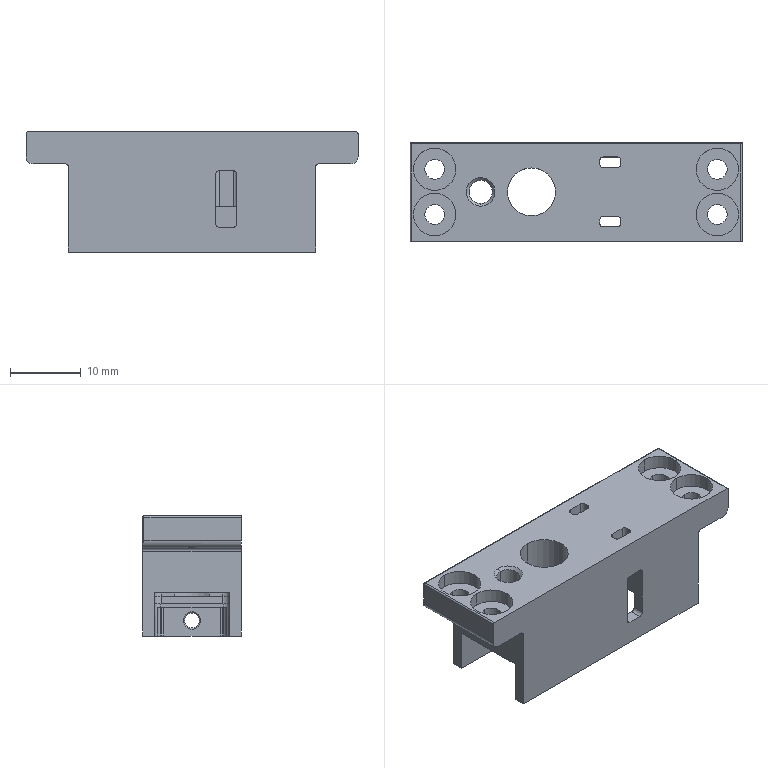NC program | NX | posted with a generic post | part box 47 x 14 x 17 mm
Lines 1 to 1495 of 12912:
N10 G17 G21 G94 G90
(FLOOR_WALL_COPY , TOOL : D63)
N12 T01 M6
N14 G54
N16 G17 G0 G90 X58. Y0. B0. C0. S6500 M3
N18 G43 Z30. H1
N20 Z5.
N22 G94 G1 Z2. F1250.
N24 X55.
N26 X-55.
N28 X-58.
N30 Z5.
N32 G0 Z30.
N34 X58.
N36 Z4.
N38 G1 Z1.
N40 X55.
N42 X-55.
N44 X-58.
N46 Z4.
N48 G0 Z30.
N50 X58.
N52 Z3.
N54 G1 Z0.
N56 X55.
N58 X-55.
N60 X-58.
N62 Z3.
N64 G0 Z30.
N66 M5
(CAVITY_MILL , TOOL : D6)
N68 T09 M6
N70 G54
N72 G17 G0 G90 X27.096 Y-2.483 B0. C0. S9500 M3
N74 G43 Z30. H9
N76 Z0.429
N78 G94 G1 Z-0.571 F1000.
N80 X24.296 Y-0.866
N82 G2 X23.796 Y0. R1.
N84 G1 Y7.002 F2200.
N86 G3 X23.501 Y7.297 R0.295
N88 G1 X21.308
N90 G3 X21.22 Y7.868 R3.82
N92 G1 Y9.997
N94 X20.5
N96 Y7.781
N98 G2 X20.6 Y7. R3.1
N100 G1 Y-7.
N102 G2 X20.3 Y-8.33 R3.1
N104 G1 Y-9.997
N106 X21.02
N108 Y-8.484
N110 G3 X21.308 Y-7.297 R3.82
N112 G1 X23.501
N114 G3 X23.796 Y-7.002 R0.295
N116 G1 Y0.
N118 G2 X24.296 Y0.866 R1.
N120 G1 X27.096 Y2.483
N122 Z0.429
N124 Y-2.483 Z-0.143 F8000.
N126 Z-1.143 F1000.
N128 X24.296 Y-0.866
N130 G2 X23.796 Y0. R1.
N132 G1 Y7.002 F2200.
N134 G3 X23.501 Y7.297 R0.295
N136 G1 X21.308
N138 G3 X21.22 Y7.868 R3.82
N140 G1 Y9.997
N142 X20.5
N144 Y7.781
N146 G2 X20.6 Y7. R3.1
N148 G1 Y-7.
N150 G2 X20.3 Y-8.33 R3.1
N152 G1 Y-9.997
N154 X21.02
N156 Y-8.484
N158 G3 X21.308 Y-7.297 R3.82
N160 G1 X23.501
N162 G3 X23.796 Y-7.002 R0.295
N164 G1 Y0.
N166 G2 X24.296 Y0.866 R1.
N168 G1 X27.096 Y2.483
N170 Z-0.143
N172 Y-2.483 Z-0.714 F8000.
N174 Z-1.714 F1000.
N176 X24.296 Y-0.866
N178 G2 X23.796 Y0. R1.
N180 G1 Y7.002 F2200.
N182 G3 X23.501 Y7.297 R0.296
N184 G1 X21.308
N186 G3 X21.22 Y7.868 R3.82
N188 G1 Y9.997
N190 X20.5
N192 Y7.781
N194 G2 X20.6 Y7. R3.1
N196 G1 Y-7.
N198 G2 X20.5 Y-7.781 R3.1
N200 G1 Y-9.997
N202 X21.22
N204 Y-7.868
N206 G3 X21.308 Y-7.297 R3.82
N208 G1 X23.501
N210 G3 X23.796 Y-7.002 R0.296
N212 G1 Y0.
N214 G2 X24.296 Y0.866 R1.
N216 G1 X27.096 Y2.483
N218 Z-0.714
N220 X27.097 Y-2.483 Z-1.286 F8000.
N222 Z-2.286 F1000.
N224 X24.297 Y-0.866
N226 G2 X23.797 Y0. R1.
N228 G1 Y7.002 F2200.
N230 G3 X23.501 Y7.297 R0.296
N232 G1 X21.308
N234 G3 X21.22 Y7.868 R3.82
N236 G1 Y9.997
N238 X20.5
N240 Y7.781
N242 G2 X20.6 Y7. R3.1
N244 G1 Y-7.
N246 G2 X20.5 Y-7.781 R3.1
N248 G1 Y-9.997
N250 X21.22
N252 Y-7.868
N254 G3 X21.308 Y-7.297 R3.82
N256 G1 X23.501
N258 G3 X23.797 Y-7.002 R0.296
N260 G1 Y0.
N262 G2 X24.297 Y0.866 R1.
N264 G1 X27.097 Y2.483
N266 Z-1.286
N268 Y-2.483 Z-1.857 F8000.
N270 Z-2.857 F1000.
N272 X24.297 Y-0.866
N274 G2 X23.797 Y0. R1.
N276 G1 Y7.002 F2200.
N278 G3 X23.501 Y7.298 R0.296
N280 G1 X21.308
N282 G3 X21.22 Y7.868 R3.82
N284 G1 Y9.998
N286 X20.5
N288 Y7.781
N290 G2 X20.6 Y7. R3.1
N292 G1 Y-7.
N294 G2 X20.5 Y-7.781 R3.1
N296 G1 Y-9.998
N298 X21.22
N300 Y-7.868
N302 G3 X21.308 Y-7.298 R3.82
N304 G1 X23.501
N306 G3 X23.797 Y-7.002 R0.296
N308 G1 Y0.
N310 G2 X24.297 Y0.866 R1.
N312 G1 X27.097 Y2.483
N314 Z-1.857
N316 Y-2.483 Z-2.429 F8000.
N318 Z-3.429 F1000.
N320 X24.297 Y-0.866
N322 G2 X23.797 Y0. R1.
N324 G1 Y7.002 F2200.
N326 G3 X23.501 Y7.298 R0.296
N328 G1 X21.308
N330 G3 X21.22 Y7.868 R3.82
N332 G1 Y9.998
N334 X20.5
N336 Y7.781
N338 G2 X20.6 Y7. R3.1
N340 G1 Y-7.
N342 G2 X20.5 Y-7.781 R3.1
N344 G1 Y-9.998
N346 X21.22
N348 Y-7.868
N350 G3 X21.308 Y-7.298 R3.82
N352 G1 X23.501
N354 G3 X23.797 Y-7.002 R0.296
N356 G1 Y0.
N358 G2 X24.297 Y0.866 R1.
N360 G1 X27.097 Y2.483
N362 Z-2.429
N364 Y-2.483 Z-3. F8000.
N366 Z-4. F1000.
N368 X24.297 Y-0.866
N370 G2 X23.797 Y0. R1.
N372 G1 Y7.002 F2200.
N374 G3 X23.501 Y7.298 R0.296
N376 G1 X21.308
N378 G3 X21.22 Y7.868 R3.82
N380 G1 Y9.998
N382 X20.5
N384 Y7.781
N386 G2 X20.6 Y7. R3.1
N388 G1 Y-7.
N390 G2 X20.5 Y-7.781 R3.1
N392 G1 Y-9.998
N394 X21.22
N396 Y-7.868
N398 G3 X21.308 Y-7.298 R3.82
N400 G1 X23.501
N402 G3 X23.797 Y-7.002 R0.296
N404 G1 Y0.
N406 G2 X24.297 Y0.866 R1.
N408 G1 X27.097 Y2.483
N410 Z-3.
N412 Y-2.483 Z-3.5 F8000.
N414 Z-4.5 F1000.
N416 X24.297 Y-0.866
N418 G2 X23.797 Y0. R1.
N420 G1 Y7.002 F2200.
N422 G3 X23.501 Y7.298 R0.296
N424 G1 X21.308
N426 G3 X21.22 Y7.868 R3.82
N428 G1 Y9.998
N430 X20.5
N432 Y7.781
N434 G2 X20.6 Y7. R3.1
N436 G1 Y-7.
N438 G2 X20.5 Y-7.781 R3.1
N440 G1 Y-9.998
N442 X21.22
N444 Y-7.868
N446 G3 X21.308 Y-7.298 R3.82
N448 G1 X23.501
N450 G3 X23.797 Y-7.002 R0.296
N452 G1 Y0.
N454 G2 X24.297 Y0.866 R1.
N456 G1 X27.097 Y2.483
N458 Z-3.5
N460 Y-2.483 Z-4. F8000.
N462 Z-5. F1000.
N464 X24.297 Y-0.866
N466 G2 X23.797 Y0. R1.
N468 G1 Y7.001 F2200.
N470 G3 X23.501 Y7.298 R0.296
N472 G1 X21.308
N474 G3 X21.22 Y7.868 R3.82
N476 G1 Y9.998
N478 X20.5
N480 Y7.781
N482 G2 X20.6 Y7. R3.1
N484 G1 Y-7.
N486 G2 X20.5 Y-7.781 R3.1
N488 G1 Y-9.998
N490 X21.22
N492 Y-7.868
N494 G3 X21.308 Y-7.298 R3.82
N496 G1 X23.501
N498 G3 X23.797 Y-7.001 R0.296
N500 G1 Y0.
N502 G2 X24.297 Y0.866 R1.
N504 G1 X27.097 Y2.483
N506 Z-4.
N508 Y-2.483 Z-4.5 F8000.
N510 Z-5.5 F1000.
N512 X24.297 Y-0.866
N514 G2 X23.797 Y0. R1.
N516 G1 Y7.001 F2200.
N518 G3 X23.501 Y7.298 R0.297
N520 G1 X21.308
N522 G3 X21.22 Y7.868 R3.82
N524 G1 Y9.998
N526 X20.5
N528 Y7.781
N530 G2 X20.6 Y7. R3.1
N532 G1 Y-7.
N534 G2 X20.5 Y-7.781 R3.1
N536 G1 Y-9.998
N538 X21.22
N540 Y-7.868
N542 G3 X21.308 Y-7.298 R3.82
N544 G1 X23.501
N546 G3 X23.797 Y-7.001 R0.297
N548 G1 Y0.
N550 G2 X24.297 Y0.866 R1.
N552 G1 X27.097 Y2.483
N554 Z-4.5
N556 Y-2.483 Z-5. F8000.
N558 Z-6. F1000.
N560 X24.297 Y-0.866
N562 G2 X23.797 Y0. R1.
N564 G1 Y7.001 F2200.
N566 G3 X23.501 Y7.298 R0.297
N568 G1 X21.308
N570 G3 X21.22 Y7.868 R3.82
N572 G1 Y9.998
N574 X20.5
N576 Y7.781
N578 G2 X20.6 Y7. R3.1
N580 G1 Y-7.
N582 G2 X20.5 Y-7.781 R3.1
N584 G1 Y-9.998
N586 X21.22
N588 Y-7.868
N590 G3 X21.308 Y-7.298 R3.82
N592 G1 X23.501
N594 G3 X23.797 Y-7.001 R0.297
N596 G1 Y0.
N598 G2 X24.297 Y0.866 R1.
N600 G1 X27.097 Y2.483
N602 Z-5.
N604 Y-2.483 Z-5.4 F8000.
N606 Z-6.4 F1000.
N608 X24.297 Y-0.866
N610 G2 X23.797 Y0. R1.
N612 G1 Y7.001 F2200.
N614 G3 X23.501 Y7.298 R0.297
N616 G1 X21.308
N618 G3 X21.22 Y7.868 R3.82
N620 G1 Y9.998
N622 X20.5
N624 Y7.781
N626 G2 X20.6 Y7. R3.1
N628 G1 Y-7.
N630 G2 X20.5 Y-7.781 R3.1
N632 G1 Y-9.998
N634 X21.22
N636 Y-7.868
N638 G3 X21.308 Y-7.298 R3.82
N640 G1 X23.501
N642 G3 X23.797 Y-7.001 R0.297
N644 G1 Y0.
N646 G2 X24.297 Y0.866 R1.
N648 G1 X27.097 Y2.483
N650 Z-5.4
N652 X27.098 Y-2.483 Z-6. F8000.
N654 Z-7. F1000.
N656 X24.298 Y-0.866
N658 G2 X23.798 Y0. R1.
N660 G1 Y7.001 F2200.
N662 G3 X23.501 Y7.298 R0.297
N664 G1 X21.308
N666 G3 X21.22 Y7.868 R3.82
N668 G1 Y9.998
N670 X20.5
N672 Y7.781
N674 G2 X20.6 Y7. R3.1
N676 G1 Y-7.
N678 G2 X20.5 Y-7.781 R3.1
N680 G1 Y-9.998
N682 X21.22
N684 Y-7.868
N686 G3 X21.308 Y-7.298 R3.82
N688 G1 X23.501
N690 G3 X23.798 Y-7.001 R0.297
N692 G1 Y0.
N694 G2 X24.298 Y0.866 R1.
N696 G1 X27.098 Y2.483
N698 Z-6.
N700 Y-2.483 Z-6.55 F8000.
N702 Z-7.55 F1000.
N704 X24.298 Y-0.866
N706 G2 X23.798 Y0. R1.
N708 G1 Y7.001 F2200.
N710 G3 X23.501 Y7.298 R0.297
N712 G1 X21.308
N714 G3 X21.22 Y7.868 R3.82
N716 G1 Y9.998
N718 X20.5
N720 Y7.781
N722 G2 X20.6 Y7. R3.1
N724 G1 Y-7.
N726 G2 X20.5 Y-7.781 R3.1
N728 G1 Y-9.998
N730 X21.22
N732 Y-7.868
N734 G3 X21.308 Y-7.298 R3.82
N736 G1 X23.501
N738 G3 X23.798 Y-7.001 R0.297
N740 G1 Y0.
N742 G2 X24.298 Y0.866 R1.
N744 G1 X27.098 Y2.483
N746 Z-6.55
N748 Y-2.483 Z-7.1 F8000.
N750 Z-8.1 F1000.
N752 X24.298 Y-0.866
N754 G2 X23.798 Y0. R1.
N756 G1 Y7.001 F2200.
N758 G3 X23.501 Y7.298 R0.297
N760 G1 X21.308
N762 G3 X21.22 Y7.868 R3.82
N764 G1 Y9.998
N766 X20.5
N768 Y7.781
N770 G2 X20.6 Y7. R3.1
N772 G1 Y-7.
N774 G2 X20.5 Y-7.781 R3.1
N776 G1 Y-9.998
N778 X21.22
N780 Y-7.868
N782 G3 X21.308 Y-7.298 R3.82
N784 G1 X23.501
N786 G3 X23.798 Y-7.001 R0.297
N788 G1 Y0.
N790 G2 X24.298 Y0.866 R1.
N792 G1 X27.098 Y2.483
N794 Z-7.1
N796 Y-2.483 Z-7.65 F8000.
N798 Z-8.65 F1000.
N800 X24.298 Y-0.866
N802 G2 X23.798 Y0. R1.
N804 G1 Y7.001 F2200.
N806 G3 X23.501 Y7.299 R0.297
N808 G1 X21.308
N810 G3 X21.22 Y7.868 R3.82
N812 G1 Y9.999
N814 X20.5
N816 Y7.781
N818 G2 X20.6 Y7. R3.1
N820 G1 Y-7.
N822 G2 X20.5 Y-7.781 R3.1
N824 G1 Y-9.999
N826 X21.22
N828 Y-7.868
N830 G3 X21.308 Y-7.299 R3.82
N832 G1 X23.501
N834 G3 X23.798 Y-7.001 R0.297
N836 G1 Y0.
N838 G2 X24.298 Y0.866 R1.
N840 G1 X27.098 Y2.483
N842 Z-7.65
N844 Y-2.483 Z-8.2 F8000.
N846 Z-9.2 F1000.
N848 X24.298 Y-0.866
N850 G2 X23.798 Y0. R1.
N852 G1 Y7.001 F2200.
N854 G3 X23.501 Y7.299 R0.298
N856 G1 X21.308
N858 G3 X21.22 Y7.868 R3.82
N860 G1 Y9.999
N862 X20.5
N864 Y7.781
N866 G2 X20.6 Y7. R3.1
N868 G1 Y-7.
N870 G2 X20.5 Y-7.781 R3.1
N872 G1 Y-9.999
N874 X21.22
N876 Y-7.868
N878 G3 X21.308 Y-7.299 R3.82
N880 G1 X23.501
N882 G3 X23.798 Y-7.001 R0.298
N884 G1 Y0.
N886 G2 X24.298 Y0.866 R1.
N888 G1 X27.098 Y2.483
N890 Z-8.2
N892 Y-2.483 Z-8.75 F8000.
N894 Z-9.75 F1000.
N896 X24.298 Y-0.866
N898 G2 X23.798 Y0. R1.
N900 G1 Y7.001 F2200.
N902 G3 X23.501 Y7.299 R0.298
N904 G1 X21.308
N906 G3 X21.22 Y7.868 R3.82
N908 G1 Y9.999
N910 X20.5
N912 Y7.781
N914 G2 X20.6 Y7. R3.1
N916 G1 Y-7.
N918 G2 X20.5 Y-7.781 R3.1
N920 G1 Y-9.999
N922 X21.22
N924 Y-7.868
N926 G3 X21.308 Y-7.299 R3.82
N928 G1 X23.501
N930 G3 X23.798 Y-7.001 R0.298
N932 G1 Y0.
N934 G2 X24.298 Y0.866 R1.
N936 G1 X27.098 Y2.483
N938 Z-8.75
N940 Y-2.483 Z-9.3 F8000.
N942 Z-10.3 F1000.
N944 X24.298 Y-0.866
N946 G2 X23.798 Y0. R1.
N948 G1 Y7.001 F2200.
N950 G3 X23.5 Y7.299 R0.298
N952 G1 X21.308
N954 G3 X21.22 Y7.868 R3.82
N956 G1 Y9.999
N958 X20.5
N960 Y7.781
N962 G2 X20.6 Y7. R3.1
N964 G1 Y-7.
N966 G2 X20.5 Y-7.781 R3.1
N968 G1 Y-9.999
N970 X21.22
N972 Y-7.868
N974 G3 X21.308 Y-7.299 R3.82
N976 G1 X23.5
N978 G3 X23.798 Y-7.001 R0.298
N980 G1 Y0.
N982 G2 X24.298 Y0.866 R1.
N984 G1 X27.098 Y2.483
N986 Z-9.3
N988 Y-2.483 Z-9.85 F8000.
N990 Z-10.85 F1000.
N992 X24.298 Y-0.866
N994 G2 X23.798 Y0. R1.
N996 G1 Y7.001 F2200.
N998 G3 X23.5 Y7.299 R0.298
N1000 G1 X21.308
N1002 G3 X21.22 Y7.868 R3.82
N1004 G1 Y9.999
N1006 X20.5
N1008 Y7.781
N1010 G2 X20.6 Y7. R3.1
N1012 G1 Y-7.
N1014 G2 X20.5 Y-7.781 R3.1
N1016 G1 Y-9.999
N1018 X21.22
N1020 Y-7.868
N1022 G3 X21.308 Y-7.299 R3.82
N1024 G1 X23.5
N1026 G3 X23.798 Y-7.001 R0.298
N1028 G1 Y0.
N1030 G2 X24.298 Y0.866 R1.
N1032 G1 X27.098 Y2.483
N1034 Z-9.85
N1036 X27.099 Y-2.483 Z-10.4 F8000.
N1038 Z-11.4 F1000.
N1040 X24.299 Y-0.866
N1042 G2 X23.799 Y0. R1.
N1044 G1 Y7.001 F2200.
N1046 G3 X23.5 Y7.299 R0.298
N1048 G1 X21.308
N1050 G3 X21.22 Y7.868 R3.82
N1052 G1 Y9.999
N1054 X20.5
N1056 Y7.781
N1058 G2 X20.6 Y7. R3.1
N1060 G1 Y-7.
N1062 G2 X20.5 Y-7.781 R3.1
N1064 G1 Y-9.999
N1066 X21.22
N1068 Y-7.868
N1070 G3 X21.308 Y-7.299 R3.82
N1072 G1 X23.5
N1074 G3 X23.799 Y-7.001 R0.298
N1076 G1 Y0.
N1078 G2 X24.299 Y0.866 R1.
N1080 G1 X27.099 Y2.483
N1082 Z-10.4
N1084 Y-2.483 Z-10.5 F8000.
N1086 Z-11.5 F1000.
N1088 X24.299 Y-0.866
N1090 G2 X23.799 Y0. R1.
N1092 G1 Y7.001 F2200.
N1094 G3 X23.5 Y7.299 R0.298
N1096 G1 X21.308
N1098 G3 X21.22 Y7.868 R3.82
N1100 G1 Y9.999
N1102 X20.5
N1104 Y7.781
N1106 G2 X20.6 Y7. R3.1
N1108 G1 Y-7.
N1110 G2 X20.5 Y-7.781 R3.1
N1112 G1 Y-9.999
N1114 X21.22
N1116 Y-7.868
N1118 G3 X21.308 Y-7.299 R3.82
N1120 G1 X23.5
N1122 G3 X23.799 Y-7.001 R0.298
N1124 G1 Y0.
N1126 G2 X24.299 Y0.866 R1.
N1128 G1 X27.099 Y2.483
N1130 Z-10.5
N1132 Y-2.483 Z-10.95 F8000.
N1134 Z-11.95 F1000.
N1136 X24.299 Y-0.866
N1138 G2 X23.799 Y0. R1.
N1140 G1 Y7.001 F2200.
N1142 G3 X23.5 Y7.299 R0.298
N1144 G1 X21.308
N1146 G3 X21.22 Y7.868 R3.82
N1148 G1 Y9.999
N1150 X20.5
N1152 Y7.781
N1154 G2 X20.6 Y7. R3.1
N1156 G1 Y-7.
N1158 G2 X20.5 Y-7.781 R3.1
N1160 G1 Y-9.999
N1162 X21.22
N1164 Y-7.868
N1166 G3 X21.308 Y-7.299 R3.82
N1168 G1 X23.5
N1170 G3 X23.799 Y-7.001 R0.298
N1172 G1 Y0.
N1174 G2 X24.299 Y0.866 R1.
N1176 G1 X27.099 Y2.483
N1178 Z-10.95
N1180 Y-2.483 Z-11.4 F8000.
N1182 Z-12.4 F1000.
N1184 X24.299 Y-0.866
N1186 G2 X23.799 Y0. R1.
N1188 G1 Y7.001 F2200.
N1190 G3 X23.5 Y7.299 R0.298
N1192 G1 X21.632
N1194 G3 X21.42 Y8.254 R3.878
N1196 G1 Y9.999
N1198 X20.7
N1200 Y8.122
N1202 G2 X20.928 Y7.002 R3.158
N1204 G1 X20.923 Y6.542
N1206 Y-6.542
N1208 X20.928 Y-7.002
N1210 G2 X20.7 Y-8.128 R3.151
N1212 G1 Y-9.999
N1214 X21.42
N1216 Y-8.26
N1218 G3 X21.633 Y-7.299 R3.871
N1220 G1 X23.5
N1222 G3 X23.799 Y-7.001 R0.298
N1224 G1 Y0.
N1226 G2 X24.299 Y0.866 R1.
N1228 G1 X27.099 Y2.483
N1230 Z-11.4
N1232 G0 Z30.
N1234 X-27.096 Y-2.483
N1236 Z0.429
N1238 G1 Z-0.571 F1000.
N1240 X-24.296 Y-0.866
N1242 G3 X-23.796 Y0. R1.
N1244 G1 X-21.096
N1246 Y-0.799 F2200.
N1248 G2 X-19.74 Y0. R5.8
N1250 X-21.096 Y0.799 R5.8
N1252 G1 Y0.
N1254 X-23.796
N1256 Y-7.002
N1258 G3 X-23.501 Y-7.297 R0.295
N1260 G1 X-21.308
N1262 G3 X-21.22 Y-7.868 R3.82
N1264 G1 Y-9.997
N1266 X-20.5
N1268 Y-7.781
N1270 G2 X-20.6 Y-7. R3.1
N1272 G1 Y-5.35
N1274 G2 X-17.5 Y-2.25 R3.1
N1276 G1 X7.606
N1278 G2 X8.387 Y-2.15 R3.1
N1280 G1 X9.162
N1282 G2 X9.433 Y-2.031 R3.1
N1284 X10.1 Y-1.575 R3.24
N1286 G1 Y1.617
N1288 X10.055 Y1.639
N1290 X10.039 Y1.607
N1292 G2 X9.433 Y2.031 R3.24
N1294 X9.162 Y2.15 R3.1
N1296 G1 X8.387
N1298 G2 X7.606 Y2.25 R3.1
N1300 G1 X-17.5
N1302 G2 X-20.6 Y5.35 R3.1
N1304 G1 Y7.
N1306 G2 X-20.5 Y7.781 R3.1
N1308 G1 Y9.997
N1310 X-21.22
N1312 Y7.868
N1314 G3 X-21.308 Y7.297 R3.82
N1316 G1 X-23.501
N1318 G3 X-23.796 Y7.002 R0.295
N1320 G1 Y0.
N1322 G2 X-24.296 Y-0.866 R1.
N1324 G1 X-27.096 Y-2.483
N1326 Z0.429
N1328 Z-0.143 F8000.
N1330 Z-1.143 F1000.
N1332 X-24.296 Y-0.866
N1334 G3 X-23.796 Y0. R1.
N1336 G1 X-21.096
N1338 Y-0.8 F2200.
N1340 G2 X-19.74 Y0. R5.8
N1342 X-21.096 Y0.8 R5.8
N1344 G1 Y0.
N1346 X-23.796
N1348 Y-7.002
N1350 G3 X-23.501 Y-7.297 R0.295
N1352 G1 X-21.308
N1354 G3 X-21.22 Y-7.868 R3.82
N1356 G1 Y-9.997
N1358 X-20.5
N1360 Y-7.781
N1362 G2 X-20.6 Y-7. R3.1
N1364 G1 Y-5.35
N1366 G2 X-17.5 Y-2.25 R3.1
N1368 G1 X7.606
N1370 G2 X8.387 Y-2.15 R3.1
N1372 G1 X9.162
N1374 G2 X9.433 Y-2.031 R3.1
N1376 X10.1 Y-1.575 R3.24
N1378 G1 Y1.617
N1380 X10.055 Y1.639
N1382 X10.039 Y1.607
N1384 G2 X9.433 Y2.031 R3.24
N1386 X9.162 Y2.15 R3.1
N1388 G1 X8.387
N1390 G2 X7.606 Y2.25 R3.1
N1392 G1 X-17.5
N1394 G2 X-20.6 Y5.35 R3.1
N1396 G1 Y7.
N1398 G2 X-20.5 Y7.781 R3.1
N1400 G1 Y9.997
N1402 X-21.22
N1404 Y7.868
N1406 G3 X-21.308 Y7.297 R3.82
N1408 G1 X-23.501
N1410 G3 X-23.796 Y7.002 R0.295
N1412 G1 Y0.
N1414 G2 X-24.296 Y-0.866 R1.
N1416 G1 X-27.096 Y-2.483
N1418 Z-0.143
N1420 Z-0.714 F8000.
N1422 Z-1.714 F1000.
N1424 X-24.296 Y-0.866
N1426 G3 X-23.796 Y0. R1.
N1428 G1 X-21.096
N1430 Y-0.8 F2200.
N1432 G2 X-19.74 Y0. R5.8
N1434 X-21.096 Y0.8 R5.8
N1436 G1 Y0.
N1438 X-23.796
N1440 Y-7.002
N1442 G3 X-23.501 Y-7.297 R0.296
N1444 G1 X-21.308
N1446 G3 X-21.22 Y-7.868 R3.82
N1448 G1 Y-9.997
N1450 X-20.5
N1452 Y-7.781
N1454 G2 X-20.6 Y-7. R3.1
N1456 G1 Y-5.35
N1458 G2 X-17.5 Y-2.25 R3.1
N1460 G1 X7.606
N1462 G2 X8.387 Y-2.15 R3.1
N1464 G1 X9.162
N1466 G2 X9.433 Y-2.031 R3.1
N1468 X10.1 Y-1.575 R3.24
N1470 G1 Y1.617
N1472 X10.055 Y1.639
N1474 X10.039 Y1.607
N1476 G2 X9.433 Y2.031 R3.24
N1478 X9.162 Y2.15 R3.1
N1480 G1 X8.387
N1482 G2 X7.606 Y2.25 R3.1
N1484 G1 X-17.5
N1486 G2 X-20.6 Y5.35 R3.1
N1488 G1 Y7.
N1490 G2 X-20.5 Y7.781 R3.1
N1492 G1 Y9.997
N1494 X-21.22
N1496 Y7.868
N1498 G3 X-21.308 Y7.297 R3.82
N1500 G1 X-23.501
N1502 G3 X-23.796 Y7.002 R0.296
N1504 G1 Y0.
N1506 G2 X-24.296 Y-0.866 R1.
N1508 G1 X-27.096 Y-2.483
N1510 Z-0.714
N1512 X-27.097 Z-1.286 F8000.
N1514 Z-2.286 F1000.
N1516 X-24.297 Y-0.866
N1518 G3 X-23.797 Y0. R1.
N1520 G1 X-21.097
N1522 Y-0.8 F2200.
N1524 G2 X-19.74 Y0. R5.8
N1526 X-21.097 Y0.8 R5.8
N1528 G1 Y0.
N1530 X-23.797
N1532 Y-7.002
N1534 G3 X-23.501 Y-7.297 R0.296
N1536 G1 X-21.308
N1538 G3 X-21.22 Y-7.868 R3.82
N1540 G1 Y-9.997
N1542 X-20.5
N1544 Y-7.781
N1546 G2 X-20.6 Y-7. R3.1
N1548 G1 Y-5.35
N1550 G2 X-17.5 Y-2.25 R3.1
N1552 G1 X7.606
N1554 G2 X8.387 Y-2.15 R3.1
N1556 G1 X9.162
N1558 G2 X9.433 Y-2.031 R3.1
N1560 X10.1 Y-1.574 R3.241
N1562 G1 Y1.617
N1564 X10.055 Y1.639
N1566 X10.039 Y1.607
N1568 G2 X9.433 Y2.031 R3.24
N1570 X9.162 Y2.15 R3.1
N1572 G1 X8.387
N1574 G2 X7.606 Y2.25 R3.1
N1576 G1 X-17.5
N1578 G2 X-20.6 Y5.35 R3.1
N1580 G1 Y7.
N1582 G2 X-20.5 Y7.781 R3.1
N1584 G1 Y9.997
N1586 X-21.22
N1588 Y7.868
N1590 G3 X-21.308 Y7.297 R3.82
N1592 G1 X-23.501
N1594 G3 X-23.797 Y7.002 R0.296
N1596 G1 Y0.
N1598 G2 X-24.297 Y-0.866 R1.
N1600 G1 X-27.097 Y-2.483
N1602 Z-1.286
N1604 Z-1.857 F8000.
N1606 Z-2.857 F1000.
N1608 X-24.297 Y-0.866
N1610 G3 X-23.797 Y0. R1.
N1612 G1 X-21.097
N1614 Y-0.8 F2200.
N1616 G2 X-19.74 Y0. R5.8
N1618 X-21.097 Y0.8 R5.8
N1620 G1 Y0.
N1622 X-23.797
N1624 Y-7.002
N1626 G3 X-23.501 Y-7.298 R0.296
N1628 G1 X-21.308
N1630 G3 X-21.22 Y-7.868 R3.82
N1632 G1 Y-9.998
N1634 X-20.5
N1636 Y-7.781
N1638 G2 X-20.6 Y-7. R3.1
N1640 G1 Y-5.35
N1642 G2 X-17.5 Y-2.25 R3.1
N1644 G1 X7.606
N1646 G2 X8.387 Y-2.15 R3.1
N1648 G1 X9.162
N1650 G2 X9.433 Y-2.031 R3.1
N1652 X10.1 Y-1.575 R3.24
N1654 G1 Y1.617
N1656 X10.055 Y1.639
N1658 X10.039 Y1.607
N1660 G2 X9.433 Y2.031 R3.24
N1662 X9.162 Y2.15 R3.1
N1664 G1 X8.387
N1666 G2 X7.606 Y2.25 R3.1
N1668 G1 X-17.5
N1670 G2 X-20.6 Y5.35 R3.1
N1672 G1 Y7.
N1674 G2 X-20.5 Y7.781 R3.1
N1676 G1 Y9.998
N1678 X-21.22
N1680 Y7.868
N1682 G3 X-21.308 Y7.298 R3.82
N1684 G1 X-23.501
N1686 G3 X-23.797 Y7.002 R0.296
N1688 G1 Y0.
N1690 G2 X-24.297 Y-0.866 R1.
N1692 G1 X-27.097 Y-2.483
N1694 Z-1.857
N1696 Z-2.429 F8000.
N1698 Z-3.429 F1000.
N1700 X-24.297 Y-0.866
N1702 G3 X-23.797 Y0. R1.
N1704 G1 X-21.097
N1706 Y-0.8 F2200.
N1708 G2 X-19.74 Y0. R5.8
N1710 X-21.097 Y0.8 R5.8
N1712 G1 Y0.
N1714 X-23.797
N1716 Y-7.002
N1718 G3 X-23.501 Y-7.298 R0.296
N1720 G1 X-21.308
N1722 G3 X-21.22 Y-7.868 R3.82
N1724 G1 Y-9.998
N1726 X-20.5
N1728 Y-7.781
N1730 G2 X-20.6 Y-7. R3.1
N1732 G1 Y-5.35
N1734 G2 X-17.5 Y-2.25 R3.1
N1736 G1 X7.606
N1738 G2 X8.387 Y-2.15 R3.1
N1740 G1 X9.162
N1742 G2 X9.433 Y-2.031 R3.1
N1744 X10.1 Y-1.575 R3.241
N1746 G1 Y1.617
N1748 X10.055 Y1.639
N1750 X10.039 Y1.607
N1752 G2 X9.433 Y2.031 R3.24
N1754 X9.162 Y2.15 R3.1
N1756 G1 X8.387
N1758 G2 X7.606 Y2.25 R3.1
N1760 G1 X-17.5
N1762 G2 X-20.6 Y5.35 R3.1
N1764 G1 Y7.
N1766 G2 X-20.5 Y7.781 R3.1
N1768 G1 Y9.998
N1770 X-21.22
N1772 Y7.868
N1774 G3 X-21.308 Y7.298 R3.82
N1776 G1 X-23.501
N1778 G3 X-23.797 Y7.002 R0.296
N1780 G1 Y0.
N1782 G2 X-24.297 Y-0.866 R1.
N1784 G1 X-27.097 Y-2.483
N1786 Z-2.429
N1788 Z-3. F8000.
N1790 Z-4. F1000.
N1792 X-24.297 Y-0.866
N1794 G3 X-23.797 Y0. R1.
N1796 G1 X-21.097
N1798 Y-0.8 F2200.
N1800 G2 X-19.74 Y0. R5.8
N1802 X-21.097 Y0.8 R5.8
N1804 G1 Y0.
N1806 X-23.797
N1808 Y-7.002
N1810 G3 X-23.501 Y-7.298 R0.296
N1812 G1 X-21.308
N1814 G3 X-21.22 Y-7.868 R3.82
N1816 G1 Y-9.998
N1818 X-20.5
N1820 Y-7.781
N1822 G2 X-20.6 Y-7. R3.1
N1824 G1 Y-5.35
N1826 G2 X-17.5 Y-2.25 R3.1
N1828 G1 X7.606
N1830 G2 X8.387 Y-2.15 R3.1
N1832 G1 X9.162
N1834 G2 X9.433 Y-2.031 R3.1
N1836 X10.1 Y-1.574 R3.241
N1838 G1 Y1.617
N1840 X10.055 Y1.639
N1842 X10.039 Y1.607
N1844 G2 X9.433 Y2.031 R3.24
N1846 X9.162 Y2.15 R3.1
N1848 G1 X8.387
N1850 G2 X7.606 Y2.25 R3.1
N1852 G1 X-17.5
N1854 G2 X-20.6 Y5.35 R3.1
N1856 G1 Y7.
N1858 G2 X-20.5 Y7.781 R3.1
N1860 G1 Y9.998
N1862 X-21.22
N1864 Y7.868
N1866 G3 X-21.308 Y7.298 R3.82
N1868 G1 X-23.501
N1870 G3 X-23.797 Y7.002 R0.296
N1872 G1 Y0.
N1874 G2 X-24.297 Y-0.866 R1.
N1876 G1 X-27.097 Y-2.483
N1878 Z-3.
N1880 Z-3.5 F8000.
N1882 Z-4.5 F1000.
N1884 X-24.297 Y-0.866
N1886 G3 X-23.797 Y0. R1.
N1888 G1 X-21.097
N1890 Y-0.8 F2200.
N1892 G2 X-19.74 Y0. R5.8
N1894 X-21.097 Y0.8 R5.8
N1896 G1 Y0.
N1898 X-23.797
N1900 Y-7.002
N1902 G3 X-23.501 Y-7.298 R0.296
N1904 G1 X-21.308
N1906 G3 X-21.22 Y-7.868 R3.82
N1908 G1 Y-9.998
N1910 X-20.5
N1912 Y-7.781
N1914 G2 X-20.6 Y-7. R3.1
N1916 G1 Y-5.35
N1918 G2 X-17.5 Y-2.25 R3.1
N1920 G1 X7.6
N1922 Y2.25
N1924 X-17.5
N1926 G2 X-20.6 Y5.35 R3.1
N1928 G1 Y7.
N1930 G2 X-20.5 Y7.781 R3.1
N1932 G1 Y9.998
N1934 X-21.22
N1936 Y7.868
N1938 G3 X-21.308 Y7.298 R3.82
N1940 G1 X-23.501
N1942 G3 X-23.797 Y7.002 R0.296
N1944 G1 Y0.
N1946 G2 X-24.297 Y-0.866 R1.
N1948 G1 X-27.097 Y-2.483
N1950 Z-3.5
N1952 X5.572 Y2.25 F8000.
N1954 X2.7 Z-3.651 F1000.
N1956 Y-2.25 Z-3.886
N1958 X7.6 Z-4.143
N1960 Y2.25 Z-4.379
N1962 X2.7 Z-4.636
N1964 Y-2.25 Z-4.872
N1966 X5.15 Z-5.
N1968 X7.6 F2200.
N1970 Y2.25
N1972 X2.7
N1974 Y-2.25
N1976 X5.15
N1978 G3 X6.016 Y-1.75 R1.
N1980 G1 Z-4.
N1982 X5.572 Y2.25 F8000.
N1984 X2.7 Z-4.151 F1000.
N1986 Y-2.25 Z-4.386
N1988 X7.6 Z-4.643
N1990 Y2.25 Z-4.879
N1992 X2.7 Z-5.136
N1994 Y-2.25 Z-5.372
N1996 X5.15 Z-5.5
N1998 X7.6 F2200.
N2000 Y2.25
N2002 X2.7
N2004 Y-2.25
N2006 X5.15
N2008 G3 X6.016 Y-1.75 R1.
N2010 G1 Z-4.5
N2012 X5.572 Y2.25 F8000.
N2014 X2.7 Z-4.651 F1000.
N2016 Y-2.25 Z-4.886
N2018 X7.6 Z-5.143
N2020 Y2.25 Z-5.379
N2022 X2.7 Z-5.636
N2024 Y-2.25 Z-5.872
N2026 X5.15 Z-6.
N2028 X7.6 F2200.
N2030 Y2.25
N2032 X2.7
N2034 Y-2.25
N2036 X5.15
N2038 G3 X6.016 Y-1.75 R1.
N2040 G1 Z-5.
N2042 X3.664 Y2.25 F8000.
N2044 X2.7 Z-5.051 F1000.
N2046 Y-2.25 Z-5.286
N2048 X7.6 Z-5.543
N2050 Y2.25 Z-5.779
N2052 X2.7 Z-6.036
N2054 Y-2.25 Z-6.272
N2056 X5.15 Z-6.4
N2058 X7.6 F2200.
N2060 Y2.25
N2062 X2.7
N2064 Y-2.25
N2066 X5.15
N2068 G3 X6.016 Y-1.75 R1.
N2070 G1 Z-5.4
N2072 G0 Z30.
N2074 X-27.097 Y-2.483
N2076 Z-4.
N2078 G1 Z-5. F1000.
N2080 X-24.297 Y-0.866
N2082 G3 X-23.797 Y0. R1.
N2084 G1 X-21.097
N2086 Y-0.8 F2200.
N2088 G2 X-19.74 Y0. R5.8
N2090 X-21.097 Y0.8 R5.8
N2092 G1 Y0.
N2094 X-23.797
N2096 Y-7.001
N2098 G3 X-23.501 Y-7.298 R0.296
N2100 G1 X-21.308
N2102 G3 X-21.22 Y-7.868 R3.82
N2104 G1 Y-9.998
N2106 X-20.5
N2108 Y-7.781
N2110 G2 X-20.6 Y-7. R3.1
N2112 G1 Y-5.35
N2114 G2 X-17.5 Y-2.25 R3.1
N2116 G1 X-5.1
N2118 Y2.25
N2120 X-17.5
N2122 G2 X-20.6 Y5.35 R3.1
N2124 G1 Y7.
N2126 G2 X-20.5 Y7.781 R3.1
N2128 G1 Y9.998
N2130 X-21.22
N2132 Y7.868
N2134 G3 X-21.308 Y7.298 R3.82
N2136 G1 X-23.501
N2138 G3 X-23.797 Y7.001 R0.296
N2140 G1 Y0.
N2142 G2 X-24.297 Y-0.866 R1.
N2144 G1 X-27.097 Y-2.483
N2146 Z-4.
N2148 Z-4.5 F8000.
N2150 Z-5.5 F1000.
N2152 X-24.297 Y-0.866
N2154 G3 X-23.797 Y0. R1.
N2156 G1 X-21.097
N2158 Y-0.8 F2200.
N2160 G2 X-19.74 Y0. R5.8
N2162 X-21.097 Y0.8 R5.8
N2164 G1 Y0.
N2166 X-23.797
N2168 Y-7.001
N2170 G3 X-23.501 Y-7.298 R0.297
N2172 G1 X-21.308
N2174 G3 X-21.22 Y-7.868 R3.82
N2176 G1 Y-9.998
N2178 X-20.5
N2180 Y-7.781
N2182 G2 X-20.6 Y-7. R3.1
N2184 G1 Y-5.35
N2186 G2 X-17.5 Y-2.25 R3.1
N2188 G1 X-5.1
N2190 Y2.25
N2192 X-17.5
N2194 G2 X-20.6 Y5.35 R3.1
N2196 G1 Y7.
N2198 G2 X-20.5 Y7.781 R3.1
N2200 G1 Y9.998
N2202 X-21.22
N2204 Y7.868
N2206 G3 X-21.308 Y7.298 R3.82
N2208 G1 X-23.501
N2210 G3 X-23.797 Y7.001 R0.297
N2212 G1 Y0.
N2214 G2 X-24.297 Y-0.866 R1.
N2216 G1 X-27.097 Y-2.483
N2218 Z-4.5
N2220 Z-5. F8000.
N2222 Z-6. F1000.
N2224 X-24.297 Y-0.866
N2226 G3 X-23.797 Y0. R1.
N2228 G1 X-21.097
N2230 Y-0.8 F2200.
N2232 G2 X-19.74 Y0. R5.8
N2234 X-21.097 Y0.8 R5.8
N2236 G1 Y0.
N2238 X-23.797
N2240 Y-7.001
N2242 G3 X-23.501 Y-7.298 R0.297
N2244 G1 X-21.308
N2246 G3 X-21.22 Y-7.868 R3.82
N2248 G1 Y-9.998
N2250 X-20.5
N2252 Y-7.781
N2254 G2 X-20.6 Y-7. R3.1
N2256 G1 Y-5.35
N2258 G2 X-17.5 Y-2.25 R3.1
N2260 G1 X-6.095
N2262 G2 X-5.495 Y-0.593 R3.1
N2264 G3 X-5.495 Y0.593 R1.
N2266 G2 X-6.095 Y2.25 R3.1
N2268 G1 X-17.5
N2270 G2 X-20.6 Y5.35 R3.1
N2272 G1 Y7.
N2274 G2 X-20.5 Y7.781 R3.1
N2276 G1 Y9.998
N2278 X-21.22
N2280 Y7.868
N2282 G3 X-21.308 Y7.298 R3.82
N2284 G1 X-23.501
N2286 G3 X-23.797 Y7.001 R0.297
N2288 G1 Y0.
N2290 G2 X-24.297 Y-0.866 R1.
N2292 G1 X-27.097 Y-2.483
N2294 Z-5.
N2296 X-21.1 Y10.598 Z-5.4 F8000.
N2298 Z-6.4 F1000.
N2300 X-20.61 Y10.065
N2302 G2 X-20.86 Y9.998 R0.5
N2304 G1 X-21.22 F2200.
N2306 Y7.868
N2308 G3 X-21.308 Y7.298 R3.82
N2310 G1 X-23.501
N2312 G3 X-23.797 Y7.001 R0.297
N2314 G1 Y-7.001
N2316 G3 X-23.501 Y-7.298 R0.297
N2318 G1 X-21.308
N2320 G3 X-21.22 Y-7.868 R3.82
N2322 G1 Y-9.998
N2324 X-20.5
N2326 Y-7.781
N2328 G2 X-20.6 Y-7. R3.1
N2330 G1 Y7.
N2332 G2 X-20.5 Y7.781 R3.1
N2334 G1 Y9.998
N2336 X-20.86
N2338 G2 X-21.726 Y10.498 R1.
N2340 G1 X-21.784 Y10.598
N2342 Z-5.4
N2344 X-21.1 Z-6. F8000.
N2346 Z-7. F1000.
N2348 X-20.61 Y10.065
N2350 G2 X-20.86 Y9.998 R0.5
N2352 G1 X-21.22 F2200.
N2354 Y7.868
N2356 G3 X-21.308 Y7.298 R3.82
N2358 G1 X-23.501
N2360 G3 X-23.798 Y7.001 R0.297
N2362 G1 Y-7.001
N2364 G3 X-23.501 Y-7.298 R0.297
N2366 G1 X-21.308
N2368 G3 X-21.22 Y-7.868 R3.82
N2370 G1 Y-9.998
N2372 X-20.5
N2374 Y-7.781
N2376 G2 X-20.6 Y-7. R3.1
N2378 G1 Y7.
N2380 G2 X-20.5 Y7.781 R3.1
N2382 G1 Y9.998
N2384 X-20.86
N2386 G2 X-21.726 Y10.498 R1.
N2388 G1 X-21.784 Y10.598
N2390 Z-6.
N2392 X-21.1 Z-6.55 F8000.
N2394 Z-7.55 F1000.
N2396 X-20.61 Y10.065
N2398 G2 X-20.86 Y9.998 R0.5
N2400 G1 X-21.22 F2200.
N2402 Y7.868
N2404 G3 X-21.308 Y7.298 R3.82
N2406 G1 X-23.501
N2408 G3 X-23.798 Y7.001 R0.297
N2410 G1 Y-7.001
N2412 G3 X-23.501 Y-7.298 R0.297
N2414 G1 X-21.308
N2416 G3 X-21.22 Y-7.868 R3.82
N2418 G1 Y-9.998
N2420 X-20.5
N2422 Y-7.781
N2424 G2 X-20.6 Y-7. R3.1
N2426 G1 Y7.
N2428 G2 X-20.5 Y7.781 R3.1
N2430 G1 Y9.998
N2432 X-20.86
N2434 G2 X-21.726 Y10.498 R1.
N2436 G1 X-21.784 Y10.598
N2438 Z-6.55
N2440 X-21.1 Z-7.1 F8000.
N2442 Z-8.1 F1000.
N2444 X-20.61 Y10.065
N2446 G2 X-20.86 Y9.998 R0.5
N2448 G1 X-21.22 F2200.
N2450 Y7.868
N2452 G3 X-21.308 Y7.298 R3.82
N2454 G1 X-23.501
N2456 G3 X-23.798 Y7.001 R0.297
N2458 G1 Y-7.001
N2460 G3 X-23.501 Y-7.298 R0.297
N2462 G1 X-21.308
N2464 G3 X-21.22 Y-7.868 R3.82
N2466 G1 Y-9.998
N2468 X-20.5
N2470 Y-7.781
N2472 G2 X-20.6 Y-7. R3.1
N2474 G1 Y7.
N2476 G2 X-20.5 Y7.781 R3.1
N2478 G1 Y9.998
N2480 X-20.86
N2482 G2 X-21.726 Y10.498 R1.
N2484 G1 X-21.784 Y10.598
N2486 Z-7.1
N2488 X-21.1 Y10.599 Z-7.65 F8000.
N2490 Z-8.65 F1000.
N2492 X-20.61 Y10.066
N2494 G2 X-20.86 Y9.999 R0.5
N2496 G1 X-21.22 F2200.
N2498 Y7.868
N2500 G3 X-21.308 Y7.299 R3.82
N2502 G1 X-23.501
N2504 G3 X-23.798 Y7.001 R0.297
N2506 G1 Y-7.001
N2508 G3 X-23.501 Y-7.299 R0.297
N2510 G1 X-21.308
N2512 G3 X-21.22 Y-7.868 R3.82
N2514 G1 Y-9.999
N2516 X-20.5
N2518 Y-7.781
N2520 G2 X-20.6 Y-7. R3.1
N2522 G1 Y7.
N2524 G2 X-20.5 Y7.781 R3.1
N2526 G1 Y9.999
N2528 X-20.86
N2530 G2 X-21.726 Y10.499 R1.
N2532 G1 X-21.784 Y10.599
N2534 Z-7.65
N2536 X-21.1 Z-8.2 F8000.
N2538 Z-9.2 F1000.
N2540 X-20.61 Y10.066
N2542 G2 X-20.86 Y9.999 R0.5
N2544 G1 X-21.22 F2200.
N2546 Y7.868
N2548 G3 X-21.308 Y7.299 R3.82
N2550 G1 X-23.501
N2552 G3 X-23.798 Y7.001 R0.298
N2554 G1 Y-7.001
N2556 G3 X-23.501 Y-7.299 R0.298
N2558 G1 X-21.308
N2560 G3 X-21.22 Y-7.868 R3.82
N2562 G1 Y-9.999
N2564 X-20.5
N2566 Y-7.781
N2568 G2 X-20.6 Y-7. R3.1
N2570 G1 Y7.
N2572 G2 X-20.5 Y7.781 R3.1
N2574 G1 Y9.999
N2576 X-20.86
N2578 G2 X-21.726 Y10.499 R1.
N2580 G1 X-21.784 Y10.599
N2582 Z-8.2
N2584 X-21.1 Z-8.75 F8000.
N2586 Z-9.75 F1000.
N2588 X-20.61 Y10.066
N2590 G2 X-20.86 Y9.999 R0.5
N2592 G1 X-21.22 F2200.
N2594 Y7.868
N2596 G3 X-21.308 Y7.299 R3.82
N2598 G1 X-23.501
N2600 G3 X-23.798 Y7.001 R0.298
N2602 G1 Y-7.001
N2604 G3 X-23.501 Y-7.299 R0.298
N2606 G1 X-21.308
N2608 G3 X-21.22 Y-7.868 R3.82
N2610 G1 Y-9.999
N2612 X-20.5
N2614 Y-7.781
N2616 G2 X-20.6 Y-7. R3.1
N2618 G1 Y7.
N2620 G2 X-20.5 Y7.781 R3.1
N2622 G1 Y9.999
N2624 X-20.86
N2626 G2 X-21.726 Y10.499 R1.
N2628 G1 X-21.784 Y10.599
N2630 Z-8.75
N2632 X-21.1 Z-9.3 F8000.
N2634 Z-10.3 F1000.
N2636 X-20.61 Y10.066
N2638 G2 X-20.86 Y9.999 R0.5
N2640 G1 X-21.22 F2200.
N2642 Y7.868
N2644 G3 X-21.308 Y7.299 R3.82
N2646 G1 X-23.5
N2648 G3 X-23.798 Y7.001 R0.298
N2650 G1 Y-7.001
N2652 G3 X-23.5 Y-7.299 R0.298
N2654 G1 X-21.308
N2656 G3 X-21.22 Y-7.868 R3.82
N2658 G1 Y-9.999
N2660 X-20.5
N2662 Y-7.781
N2664 G2 X-20.6 Y-7. R3.1
N2666 G1 Y7.
N2668 G2 X-20.5 Y7.781 R3.1
N2670 G1 Y9.999
N2672 X-20.86
N2674 G2 X-21.726 Y10.499 R1.
N2676 G1 X-21.784 Y10.599
N2678 Z-9.3
N2680 X-21.1 Z-9.85 F8000.
N2682 Z-10.85 F1000.
N2684 X-20.61 Y10.066
N2686 G2 X-20.86 Y9.999 R0.5
N2688 G1 X-21.22 F2200.
N2690 Y7.868
N2692 G3 X-21.308 Y7.299 R3.82
N2694 G1 X-23.5
N2696 G3 X-23.798 Y7.001 R0.298
N2698 G1 Y-7.001
N2700 G3 X-23.5 Y-7.299 R0.298
N2702 G1 X-21.308
N2704 G3 X-21.22 Y-7.868 R3.82
N2706 G1 Y-9.999
N2708 X-20.5
N2710 Y-7.781
N2712 G2 X-20.6 Y-7. R3.1
N2714 G1 Y7.
N2716 G2 X-20.5 Y7.781 R3.1
N2718 G1 Y9.999
N2720 X-20.86
N2722 G2 X-21.726 Y10.499 R1.
N2724 G1 X-21.784 Y10.599
N2726 Z-9.85
N2728 X-21.1 Z-10.4 F8000.
N2730 Z-11.4 F1000.
N2732 X-20.61 Y10.066
N2734 G2 X-20.86 Y9.999 R0.5
N2736 G1 X-21.22 F2200.
N2738 Y7.868
N2740 G3 X-21.308 Y7.299 R3.82
N2742 G1 X-23.5
N2744 G3 X-23.799 Y7.001 R0.298
N2746 G1 Y-7.001
N2748 G3 X-23.5 Y-7.299 R0.298
N2750 G1 X-21.308
N2752 G3 X-21.22 Y-7.868 R3.82
N2754 G1 Y-9.999
N2756 X-20.5
N2758 Y-7.781
N2760 G2 X-20.6 Y-7. R3.1
N2762 G1 Y7.
N2764 G2 X-20.5 Y7.781 R3.1
N2766 G1 Y9.999
N2768 X-20.86
N2770 G2 X-21.726 Y10.499 R1.
N2772 G1 X-21.784 Y10.599
N2774 Z-10.4
N2776 X-21.1 Z-10.5 F8000.
N2778 Z-11.5 F1000.
N2780 X-20.61 Y10.066
N2782 G2 X-20.86 Y9.999 R0.5
N2784 G1 X-21.22 F2200.
N2786 Y7.868
N2788 G3 X-21.308 Y7.299 R3.82
N2790 G1 X-23.5
N2792 G3 X-23.799 Y7.001 R0.298
N2794 G1 Y-7.001
N2796 G3 X-23.5 Y-7.299 R0.298
N2798 G1 X-21.308
N2800 G3 X-21.22 Y-7.868 R3.82
N2802 G1 Y-9.999
N2804 X-20.5
N2806 Y-7.781
N2808 G2 X-20.6 Y-7. R3.1
N2810 G1 Y7.
N2812 G2 X-20.5 Y7.781 R3.1
N2814 G1 Y9.999
N2816 X-20.86
N2818 G2 X-21.726 Y10.499 R1.
N2820 G1 X-21.784 Y10.599
N2822 Z-10.5
N2824 X-21.1 Z-10.95 F8000.
N2826 Z-11.95 F1000.
N2828 X-20.61 Y10.066
N2830 G2 X-20.86 Y9.999 R0.5
N2832 G1 X-21.22 F2200.
N2834 Y7.868
N2836 G3 X-21.308 Y7.299 R3.82
N2838 G1 X-23.5
N2840 G3 X-23.799 Y7.001 R0.298
N2842 G1 Y-7.001
N2844 G3 X-23.5 Y-7.299 R0.298
N2846 G1 X-21.308
N2848 G3 X-21.22 Y-7.868 R3.82
N2850 G1 Y-9.999
N2852 X-20.5
N2854 Y-7.781
N2856 G2 X-20.6 Y-7. R3.1
N2858 G1 Y7.
N2860 G2 X-20.5 Y7.781 R3.1
N2862 G1 Y9.999
N2864 X-20.86
N2866 G2 X-21.726 Y10.499 R1.
N2868 G1 X-21.784 Y10.599
N2870 Z-10.95
N2872 X-21.3 Z-11.4 F8000.
N2874 Z-12.4 F1000.
N2876 X-20.793 Y9.749
N2878 G2 X-20.86 Y9.999 R0.5
N2880 G1 X-21.42 F2200.
N2882 Y8.239
N2884 G3 X-21.627 Y7.299 R3.88
N2886 G1 X-23.5
N2888 G3 X-23.799 Y7.001 R0.298
N2890 G1 Y-7.001
N2892 G3 X-23.5 Y-7.299 R0.298
N2894 G1 X-21.633
N2896 G3 X-21.42 Y-8.259 R3.868
N2898 G1 Y-9.999
N2900 X-20.7
N2902 Y-8.126
N2904 G2 X-20.928 Y-7.002 R3.148
N2906 G1 X-20.923 Y-6.542
N2908 Y7.
N2910 G2 X-20.7 Y8.108 R3.16
N2912 G1 Y9.999
N2914 X-20.86
N2916 G2 X-21.726 Y10.499 R1.
N2918 G1 X-21.784 Y10.599
N2920 Z-11.4
N2922 G0 Z30.
(HOLE_MILLING_COPY , TOOL : D6)
N2924 X-6.3 Y0.
N2926 Z-5.1
N2928 G3 X-5.75 Y-0.55 R0.55 F1300.
N2930 X-5.2 Y0. R0.55
N2932 X-5.2 Y0. Z-5.5 I-1.1 J0.
N2934 X-5.2 Y0. Z-5.9 I-1.1 J0.
N2936 X-5.2 Y0. Z-6.3 I-1.1 J0.
N2938 X-5.2 Y0. Z-6.7 I-1.1 J0.
N2940 X-5.2 Y0. Z-7.1 I-1.1 J0.
N2942 X-5.2 Y0. Z-7.5 I-1.1 J0.
N2944 X-5.2 Y0. Z-7.9 I-1.1 J0.
N2946 X-5.2 Y0. Z-8.3 I-1.1 J0.
N2948 X-5.2 Y0. Z-8.7 I-1.1 J0.
N2950 X-5.2 Y0. Z-9.1 I-1.1 J0.
N2952 X-5.2 Y0. Z-9.5 I-1.1 J0.
N2954 X-5.2 Y0. Z-9.9 I-1.1 J0.
N2956 X-5.2 Y0. Z-10.3 I-1.1 J0.
N2958 X-5.2 Y0. Z-10.7 I-1.1 J0.
N2960 X-5.2 Y0. Z-11.1 I-1.1 J0.
N2962 X-5.2 Y0. Z-11.5 I-1.1 J0.
N2964 X-6.3 Y1.1 Z-11.6 R1.1
N2966 X-7.4 Y0. R1.1
N2968 X-6.3 Y1.1 R-1.1
N2970 X-6.85 Y0.55 R0.55
N2972 X-6.3 Y0. R0.55
N2974 G0 Z30.
N2976 M5